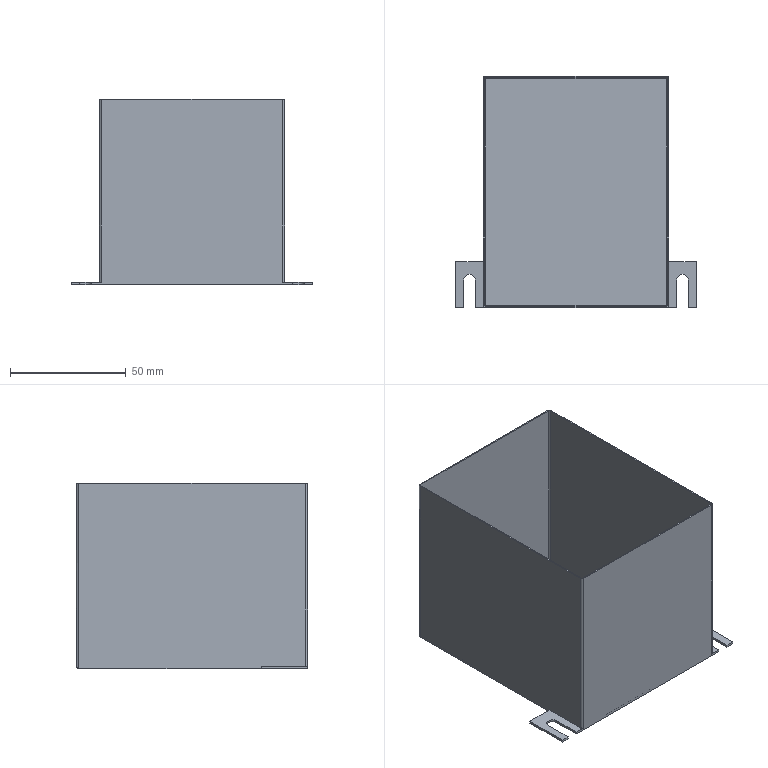Part | NX | features BREP 1 | 1 solid | 42 faces | box 104 x 100 x 80 mm | volume 18522 mm3 | plane 23 | cylinder 15 | sphere 4 | commonest cylinder face diameters 1 x8 2 x5 5 x2
STEP:
#1=CARTESIAN_POINT('',(48.5,-50.,0.));
#2=VERTEX_POINT('',#1);
#3=CARTESIAN_POINT('',(48.5,-50.,1.));
#4=VERTEX_POINT('',#3);
#5=CARTESIAN_POINT('',(48.5,-50.,-0.00005));
#6=DIRECTION('',(0.,0.,1.));
#7=VECTOR('',#6,1000.);
#8=LINE('',#5,#7);
#9=EDGE_CURVE('',#2,#4,#8,.T.);
#10=ORIENTED_EDGE('',*,*,#9,.F.);
#11=CARTESIAN_POINT('',(52.,-50.,0.));
#12=VERTEX_POINT('',#11);
#13=CARTESIAN_POINT('',(-40.,-50.,0.));
#14=DIRECTION('',(1.,0.,0.));
#15=VECTOR('',#14,1000.);
#16=LINE('',#13,#15);
#17=EDGE_CURVE('',#2,#12,#16,.T.);
#18=ORIENTED_EDGE('',*,*,#17,.T.);
#19=CARTESIAN_POINT('',(52.,-50.,1.));
#20=VERTEX_POINT('',#19);
#21=CARTESIAN_POINT('',(52.,-50.,0.));
#22=DIRECTION('',(0.,0.,1.));
#23=VECTOR('',#22,1000.);
#24=LINE('',#21,#23);
#25=EDGE_CURVE('',#12,#20,#24,.T.);
#26=ORIENTED_EDGE('',*,*,#25,.T.);
#27=CARTESIAN_POINT('',(52.,-50.,1.));
#28=DIRECTION('',(-1.,0.,0.));
#29=VECTOR('',#28,1000.);
#30=LINE('',#27,#29);
#31=EDGE_CURVE('',#20,#4,#30,.T.);
#32=ORIENTED_EDGE('',*,*,#31,.T.);
#33=EDGE_LOOP('',(#10,#18,#26,#32));
#34=FACE_BOUND('',#33,.T.);
#35=CARTESIAN_POINT('',(-40.,-50.,80.));
#36=DIRECTION('',(0.,1.,0.));
#37=DIRECTION('',(1.,0.,0.));
#38=AXIS2_PLACEMENT_3D('',#35,#36,#37);
#39=PLANE('',#38);
#40=ADVANCED_FACE('',(#34),#39,.F.);
#41=CARTESIAN_POINT('',(43.5,-50.,1.));
#42=VERTEX_POINT('',#41);
#43=CARTESIAN_POINT('',(39.,-50.,1.));
#44=VERTEX_POINT('',#43);
#45=CARTESIAN_POINT('',(52.,-50.,1.));
#46=DIRECTION('',(-1.,0.,0.));
#47=VECTOR('',#46,1000.);
#48=LINE('',#45,#47);
#49=EDGE_CURVE('',#42,#44,#48,.T.);
#50=ORIENTED_EDGE('',*,*,#49,.T.);
#51=CARTESIAN_POINT('',(39.,-50.,80.));
#52=VERTEX_POINT('',#51);
#53=CARTESIAN_POINT('',(39.,-50.,80.));
#54=DIRECTION('',(0.,0.,1.));
#55=VECTOR('',#54,1000.);
#56=LINE('',#53,#55);
#57=EDGE_CURVE('',#44,#52,#56,.T.);
#58=ORIENTED_EDGE('',*,*,#57,.T.);
#59=CARTESIAN_POINT('',(-39.,-50.,80.));
#60=VERTEX_POINT('',#59);
#61=CARTESIAN_POINT('',(-40.,-50.,80.));
#62=DIRECTION('',(1.,0.,0.));
#63=VECTOR('',#62,1000.);
#64=LINE('',#61,#63);
#65=EDGE_CURVE('',#60,#52,#64,.T.);
#66=ORIENTED_EDGE('',*,*,#65,.F.);
#67=CARTESIAN_POINT('',(-39.,-50.,1.));
#68=VERTEX_POINT('',#67);
#69=CARTESIAN_POINT('',(-39.,-50.,80.));
#70=DIRECTION('',(0.,0.,-1.));
#71=VECTOR('',#70,1000.);
#72=LINE('',#69,#71);
#73=EDGE_CURVE('',#60,#68,#72,.T.);
#74=ORIENTED_EDGE('',*,*,#73,.T.);
#75=CARTESIAN_POINT('',(-43.5,-50.,1.));
#76=VERTEX_POINT('',#75);
#77=CARTESIAN_POINT('',(-52.,-50.,1.));
#78=DIRECTION('',(1.,0.,0.));
#79=VECTOR('',#78,1000.);
#80=LINE('',#77,#79);
#81=EDGE_CURVE('',#76,#68,#80,.T.);
#82=ORIENTED_EDGE('',*,*,#81,.F.);
#83=CARTESIAN_POINT('',(-43.5,-50.,0.));
#84=VERTEX_POINT('',#83);
#85=CARTESIAN_POINT('',(-43.5,-50.,-0.00005));
#86=DIRECTION('',(0.,0.,1.));
#87=VECTOR('',#86,1000.);
#88=LINE('',#85,#87);
#89=EDGE_CURVE('',#84,#76,#88,.T.);
#90=ORIENTED_EDGE('',*,*,#89,.F.);
#91=CARTESIAN_POINT('',(43.5,-50.,0.));
#92=VERTEX_POINT('',#91);
#93=CARTESIAN_POINT('',(-40.,-50.,0.));
#94=DIRECTION('',(1.,0.,0.));
#95=VECTOR('',#94,1000.);
#96=LINE('',#93,#95);
#97=EDGE_CURVE('',#84,#92,#96,.T.);
#98=ORIENTED_EDGE('',*,*,#97,.T.);
#99=CARTESIAN_POINT('',(43.5,-50.,-0.00005));
#100=DIRECTION('',(0.,0.,1.));
#101=VECTOR('',#100,1000.);
#102=LINE('',#99,#101);
#103=EDGE_CURVE('',#92,#42,#102,.T.);
#104=ORIENTED_EDGE('',*,*,#103,.T.);
#105=EDGE_LOOP('',(#50,#58,#66,#74,#82,#90,#98,#104));
#106=FACE_BOUND('',#105,.T.);
#107=CARTESIAN_POINT('',(-40.,-50.,80.));
#108=DIRECTION('',(0.,1.,0.));
#109=DIRECTION('',(1.,0.,0.));
#110=AXIS2_PLACEMENT_3D('',#107,#108,#109);
#111=PLANE('',#110);
#112=ADVANCED_FACE('',(#106),#111,.F.);
#113=CARTESIAN_POINT('',(-40.,49.,0.));
#114=VERTEX_POINT('',#113);
#115=CARTESIAN_POINT('',(-40.,-30.,0.));
#116=VERTEX_POINT('',#115);
#117=CARTESIAN_POINT('',(-40.,-50.,0.));
#118=DIRECTION('',(0.,-1.,0.));
#119=VECTOR('',#118,1000.);
#120=LINE('',#117,#119);
#121=EDGE_CURVE('',#114,#116,#120,.T.);
#122=ORIENTED_EDGE('',*,*,#121,.F.);
#123=CARTESIAN_POINT('',(40.,49.,0.));
#124=VERTEX_POINT('',#123);
#125=CARTESIAN_POINT('',(40.,49.,0.));
#126=DIRECTION('',(1.,0.,0.));
#127=VECTOR('',#126,1000.);
#128=LINE('',#125,#127);
#129=EDGE_CURVE('',#114,#124,#128,.T.);
#130=ORIENTED_EDGE('',*,*,#129,.T.);
#131=CARTESIAN_POINT('',(40.,-30.,0.));
#132=VERTEX_POINT('',#131);
#133=CARTESIAN_POINT('',(40.,-50.,0.));
#134=DIRECTION('',(0.,1.,0.));
#135=VECTOR('',#134,1000.);
#136=LINE('',#133,#135);
#137=EDGE_CURVE('',#132,#124,#136,.T.);
#138=ORIENTED_EDGE('',*,*,#137,.F.);
#139=CARTESIAN_POINT('',(52.,-30.,0.));
#140=VERTEX_POINT('',#139);
#141=CARTESIAN_POINT('',(52.,-30.,0.));
#142=DIRECTION('',(-1.,0.,0.));
#143=VECTOR('',#142,1000.);
#144=LINE('',#141,#143);
#145=EDGE_CURVE('',#140,#132,#144,.T.);
#146=ORIENTED_EDGE('',*,*,#145,.F.);
#147=CARTESIAN_POINT('',(52.,-50.,0.));
#148=DIRECTION('',(0.,-1.,0.));
#149=VECTOR('',#148,1000.);
#150=LINE('',#147,#149);
#151=EDGE_CURVE('',#140,#12,#150,.T.);
#152=ORIENTED_EDGE('',*,*,#151,.T.);
#153=ORIENTED_EDGE('',*,*,#17,.F.);
#154=CARTESIAN_POINT('',(48.5,-38.,0.));
#155=VERTEX_POINT('',#154);
#156=CARTESIAN_POINT('',(48.5,0.,0.));
#157=DIRECTION('',(0.,1.,0.));
#158=VECTOR('',#157,1000.);
#159=LINE('',#156,#158);
#160=EDGE_CURVE('',#2,#155,#159,.T.);
#161=ORIENTED_EDGE('',*,*,#160,.T.);
#162=CARTESIAN_POINT('',(43.5,-38.,0.));
#163=VERTEX_POINT('',#162);
#164=CARTESIAN_POINT('',(46.,-38.,0.));
#165=DIRECTION('',(0.,0.,1.));
#166=DIRECTION('',(-1.,0.,0.));
#167=AXIS2_PLACEMENT_3D('',#164,#165,#166);
#168=CIRCLE('',#167,2.5);
#169=EDGE_CURVE('',#155,#163,#168,.T.);
#170=ORIENTED_EDGE('',*,*,#169,.T.);
#171=CARTESIAN_POINT('',(43.5,0.,0.));
#172=DIRECTION('',(0.,-1.,0.));
#173=VECTOR('',#172,1000.);
#174=LINE('',#171,#173);
#175=EDGE_CURVE('',#163,#92,#174,.T.);
#176=ORIENTED_EDGE('',*,*,#175,.T.);
#177=ORIENTED_EDGE('',*,*,#97,.F.);
#178=CARTESIAN_POINT('',(-43.5,-38.,0.));
#179=VERTEX_POINT('',#178);
#180=CARTESIAN_POINT('',(-43.5,0.,0.));
#181=DIRECTION('',(0.,-1.,0.));
#182=VECTOR('',#181,1000.);
#183=LINE('',#180,#182);
#184=EDGE_CURVE('',#179,#84,#183,.T.);
#185=ORIENTED_EDGE('',*,*,#184,.F.);
#186=CARTESIAN_POINT('',(-48.5,-38.,0.));
#187=VERTEX_POINT('',#186);
#188=CARTESIAN_POINT('',(-46.,-38.,0.));
#189=DIRECTION('',(0.,0.,-1.));
#190=DIRECTION('',(-1.,0.,0.));
#191=AXIS2_PLACEMENT_3D('',#188,#189,#190);
#192=CIRCLE('',#191,2.5);
#193=EDGE_CURVE('',#187,#179,#192,.T.);
#194=ORIENTED_EDGE('',*,*,#193,.F.);
#195=CARTESIAN_POINT('',(-48.5,-50.,0.));
#196=VERTEX_POINT('',#195);
#197=CARTESIAN_POINT('',(-48.5,0.,0.));
#198=DIRECTION('',(0.,1.,0.));
#199=VECTOR('',#198,1000.);
#200=LINE('',#197,#199);
#201=EDGE_CURVE('',#196,#187,#200,.T.);
#202=ORIENTED_EDGE('',*,*,#201,.F.);
#203=CARTESIAN_POINT('',(-52.,-50.,0.));
#204=VERTEX_POINT('',#203);
#205=CARTESIAN_POINT('',(-40.,-50.,0.));
#206=DIRECTION('',(1.,0.,0.));
#207=VECTOR('',#206,1000.);
#208=LINE('',#205,#207);
#209=EDGE_CURVE('',#204,#196,#208,.T.);
#210=ORIENTED_EDGE('',*,*,#209,.F.);
#211=CARTESIAN_POINT('',(-52.,-30.,0.));
#212=VERTEX_POINT('',#211);
#213=CARTESIAN_POINT('',(-52.,-50.,0.));
#214=DIRECTION('',(0.,-1.,0.));
#215=VECTOR('',#214,1000.);
#216=LINE('',#213,#215);
#217=EDGE_CURVE('',#212,#204,#216,.T.);
#218=ORIENTED_EDGE('',*,*,#217,.F.);
#219=CARTESIAN_POINT('',(-52.,-30.,0.));
#220=DIRECTION('',(1.,0.,0.));
#221=VECTOR('',#220,1000.);
#222=LINE('',#219,#221);
#223=EDGE_CURVE('',#212,#116,#222,.T.);
#224=ORIENTED_EDGE('',*,*,#223,.T.);
#225=EDGE_LOOP('',(#122,#130,#138,#146,#152,#153,#161,#170,#176,#177,#185,#194,#202,#210,#218,#224));
#226=FACE_BOUND('',#225,.T.);
#227=CARTESIAN_POINT('',(0.,0.,0.));
#228=DIRECTION('',(0.,0.,-1.));
#229=DIRECTION('',(0.,-1.,0.));
#230=AXIS2_PLACEMENT_3D('',#227,#228,#229);
#231=PLANE('',#230);
#232=ADVANCED_FACE('',(#226),#231,.T.);
#233=CARTESIAN_POINT('',(43.5,-38.,1.));
#234=VERTEX_POINT('',#233);
#235=CARTESIAN_POINT('',(48.5,-38.,1.));
#236=VERTEX_POINT('',#235);
#237=CARTESIAN_POINT('',(46.,-38.,1.));
#238=DIRECTION('',(0.,0.,-1.));
#239=DIRECTION('',(-1.,0.,0.));
#240=AXIS2_PLACEMENT_3D('',#237,#238,#239);
#241=CIRCLE('',#240,2.5);
#242=EDGE_CURVE('',#234,#236,#241,.T.);
#243=ORIENTED_EDGE('',*,*,#242,.T.);
#244=CARTESIAN_POINT('',(48.5,-38.,1.));
#245=DIRECTION('',(0.,-1.,0.));
#246=VECTOR('',#245,1000.);
#247=LINE('',#244,#246);
#248=EDGE_CURVE('',#236,#4,#247,.T.);
#249=ORIENTED_EDGE('',*,*,#248,.T.);
#250=ORIENTED_EDGE('',*,*,#31,.F.);
#251=CARTESIAN_POINT('',(52.,-30.,1.));
#252=VERTEX_POINT('',#251);
#253=CARTESIAN_POINT('',(52.,-50.,1.));
#254=DIRECTION('',(0.,1.,0.));
#255=VECTOR('',#254,1000.);
#256=LINE('',#253,#255);
#257=EDGE_CURVE('',#20,#252,#256,.T.);
#258=ORIENTED_EDGE('',*,*,#257,.T.);
#259=CARTESIAN_POINT('',(40.,-30.,1.));
#260=VERTEX_POINT('',#259);
#261=CARTESIAN_POINT('',(52.,-30.,1.));
#262=DIRECTION('',(-1.,0.,0.));
#263=VECTOR('',#262,1000.);
#264=LINE('',#261,#263);
#265=EDGE_CURVE('',#252,#260,#264,.T.);
#266=ORIENTED_EDGE('',*,*,#265,.T.);
#267=CARTESIAN_POINT('',(40.,-49.,1.));
#268=VERTEX_POINT('',#267);
#269=CARTESIAN_POINT('',(40.,-50.,1.));
#270=DIRECTION('',(0.,1.,0.));
#271=VECTOR('',#270,1000.);
#272=LINE('',#269,#271);
#273=EDGE_CURVE('',#268,#260,#272,.T.);
#274=ORIENTED_EDGE('',*,*,#273,.F.);
#275=CARTESIAN_POINT('',(39.,-49.,1.));
#276=DIRECTION('',(0.,0.,-1.));
#277=DIRECTION('',(1.,0.,0.));
#278=AXIS2_PLACEMENT_3D('',#275,#276,#277);
#279=CIRCLE('',#278,1.);
#280=EDGE_CURVE('',#268,#44,#279,.T.);
#281=ORIENTED_EDGE('',*,*,#280,.T.);
#282=ORIENTED_EDGE('',*,*,#49,.F.);
#283=CARTESIAN_POINT('',(43.5,-38.,1.));
#284=DIRECTION('',(0.,1.,0.));
#285=VECTOR('',#284,1000.);
#286=LINE('',#283,#285);
#287=EDGE_CURVE('',#42,#234,#286,.T.);
#288=ORIENTED_EDGE('',*,*,#287,.T.);
#289=EDGE_LOOP('',(#243,#249,#250,#258,#266,#274,#281,#282,#288));
#290=FACE_BOUND('',#289,.T.);
#291=CARTESIAN_POINT('',(52.,-50.,1.));
#292=DIRECTION('',(0.,0.,1.));
#293=DIRECTION('',(1.,0.,0.));
#294=AXIS2_PLACEMENT_3D('',#291,#292,#293);
#295=PLANE('',#294);
#296=ADVANCED_FACE('',(#290),#295,.T.);
#297=CARTESIAN_POINT('',(-40.,-49.,1.));
#298=VERTEX_POINT('',#297);
#299=CARTESIAN_POINT('',(-40.,-30.,1.));
#300=VERTEX_POINT('',#299);
#301=CARTESIAN_POINT('',(-40.,-50.,1.));
#302=DIRECTION('',(0.,1.,0.));
#303=VECTOR('',#302,1000.);
#304=LINE('',#301,#303);
#305=EDGE_CURVE('',#298,#300,#304,.T.);
#306=ORIENTED_EDGE('',*,*,#305,.F.);
#307=CARTESIAN_POINT('',(-40.,-49.,80.));
#308=VERTEX_POINT('',#307);
#309=CARTESIAN_POINT('',(-40.,-49.,80.));
#310=DIRECTION('',(0.,0.,1.));
#311=VECTOR('',#310,1000.);
#312=LINE('',#309,#311);
#313=EDGE_CURVE('',#298,#308,#312,.T.);
#314=ORIENTED_EDGE('',*,*,#313,.T.);
#315=CARTESIAN_POINT('',(-40.,49.,80.));
#316=VERTEX_POINT('',#315);
#317=CARTESIAN_POINT('',(-40.,-50.,80.));
#318=DIRECTION('',(0.,-1.,0.));
#319=VECTOR('',#318,1000.);
#320=LINE('',#317,#319);
#321=EDGE_CURVE('',#316,#308,#320,.T.);
#322=ORIENTED_EDGE('',*,*,#321,.F.);
#323=CARTESIAN_POINT('',(-40.,49.,80.));
#324=DIRECTION('',(0.,0.,-1.));
#325=VECTOR('',#324,1000.);
#326=LINE('',#323,#325);
#327=EDGE_CURVE('',#316,#114,#326,.T.);
#328=ORIENTED_EDGE('',*,*,#327,.T.);
#329=ORIENTED_EDGE('',*,*,#121,.T.);
#330=CARTESIAN_POINT('',(-40.,-30.,0.));
#331=DIRECTION('',(0.,0.,-1.));
#332=VECTOR('',#331,1000.);
#333=LINE('',#330,#332);
#334=EDGE_CURVE('',#300,#116,#333,.T.);
#335=ORIENTED_EDGE('',*,*,#334,.F.);
#336=EDGE_LOOP('',(#306,#314,#322,#328,#329,#335));
#337=FACE_BOUND('',#336,.T.);
#338=CARTESIAN_POINT('',(-40.,-50.,80.));
#339=DIRECTION('',(1.,0.,0.));
#340=DIRECTION('',(0.,1.,0.));
#341=AXIS2_PLACEMENT_3D('',#338,#339,#340);
#342=PLANE('',#341);
#343=ADVANCED_FACE('',(#337),#342,.F.);
#344=CARTESIAN_POINT('',(40.,-49.,80.));
#345=VERTEX_POINT('',#344);
#346=CARTESIAN_POINT('',(40.,49.,80.));
#347=VERTEX_POINT('',#346);
#348=CARTESIAN_POINT('',(40.,-50.,80.));
#349=DIRECTION('',(0.,1.,0.));
#350=VECTOR('',#349,1000.);
#351=LINE('',#348,#350);
#352=EDGE_CURVE('',#345,#347,#351,.T.);
#353=ORIENTED_EDGE('',*,*,#352,.T.);
#354=CARTESIAN_POINT('',(39.,50.,80.));
#355=VERTEX_POINT('',#354);
#356=CARTESIAN_POINT('',(39.,49.,80.));
#357=DIRECTION('',(0.,0.,1.));
#358=DIRECTION('',(-1.,0.,0.));
#359=AXIS2_PLACEMENT_3D('',#356,#357,#358);
#360=CIRCLE('',#359,1.);
#361=EDGE_CURVE('',#347,#355,#360,.T.);
#362=ORIENTED_EDGE('',*,*,#361,.T.);
#363=CARTESIAN_POINT('',(-39.,50.,80.));
#364=VERTEX_POINT('',#363);
#365=CARTESIAN_POINT('',(-40.,50.,80.));
#366=DIRECTION('',(-1.,0.,0.));
#367=VECTOR('',#366,1000.);
#368=LINE('',#365,#367);
#369=EDGE_CURVE('',#355,#364,#368,.T.);
#370=ORIENTED_EDGE('',*,*,#369,.T.);
#371=CARTESIAN_POINT('',(-39.,49.,80.));
#372=DIRECTION('',(0.,0.,1.));
#373=DIRECTION('',(-1.,0.,0.));
#374=AXIS2_PLACEMENT_3D('',#371,#372,#373);
#375=CIRCLE('',#374,1.);
#376=EDGE_CURVE('',#364,#316,#375,.T.);
#377=ORIENTED_EDGE('',*,*,#376,.T.);
#378=ORIENTED_EDGE('',*,*,#321,.T.);
#379=CARTESIAN_POINT('',(-39.,-49.,80.));
#380=DIRECTION('',(0.,0.,1.));
#381=DIRECTION('',(-1.,0.,0.));
#382=AXIS2_PLACEMENT_3D('',#379,#380,#381);
#383=CIRCLE('',#382,1.);
#384=EDGE_CURVE('',#308,#60,#383,.T.);
#385=ORIENTED_EDGE('',*,*,#384,.T.);
#386=ORIENTED_EDGE('',*,*,#65,.T.);
#387=CARTESIAN_POINT('',(39.,-49.,80.));
#388=DIRECTION('',(0.,0.,1.));
#389=DIRECTION('',(-1.,0.,0.));
#390=AXIS2_PLACEMENT_3D('',#387,#388,#389);
#391=CIRCLE('',#390,1.);
#392=EDGE_CURVE('',#52,#345,#391,.T.);
#393=ORIENTED_EDGE('',*,*,#392,.T.);
#394=EDGE_LOOP('',(#353,#362,#370,#377,#378,#385,#386,#393));
#395=FACE_BOUND('',#394,.T.);
#396=CARTESIAN_POINT('',(39.5,-49.,80.));
#397=VERTEX_POINT('',#396);
#398=CARTESIAN_POINT('',(39.5,49.,80.));
#399=VERTEX_POINT('',#398);
#400=CARTESIAN_POINT('',(39.5,0.,80.));
#401=DIRECTION('',(0.,1.,0.));
#402=VECTOR('',#401,1000.);
#403=LINE('',#400,#402);
#404=EDGE_CURVE('',#397,#399,#403,.T.);
#405=ORIENTED_EDGE('',*,*,#404,.F.);
#406=CARTESIAN_POINT('',(39.,-49.5,80.));
#407=VERTEX_POINT('',#406);
#408=CARTESIAN_POINT('',(39.,-49.,80.));
#409=DIRECTION('',(0.,0.,-1.));
#410=DIRECTION('',(-1.,0.,0.));
#411=AXIS2_PLACEMENT_3D('',#408,#409,#410);
#412=CIRCLE('',#411,0.5);
#413=EDGE_CURVE('',#397,#407,#412,.T.);
#414=ORIENTED_EDGE('',*,*,#413,.T.);
#415=CARTESIAN_POINT('',(-39.,-49.5,80.));
#416=VERTEX_POINT('',#415);
#417=CARTESIAN_POINT('',(0.,-49.5,80.));
#418=DIRECTION('',(1.,0.,0.));
#419=VECTOR('',#418,1000.);
#420=LINE('',#417,#419);
#421=EDGE_CURVE('',#416,#407,#420,.T.);
#422=ORIENTED_EDGE('',*,*,#421,.F.);
#423=CARTESIAN_POINT('',(-39.5,-49.,80.));
#424=VERTEX_POINT('',#423);
#425=CARTESIAN_POINT('',(-39.,-49.,80.));
#426=DIRECTION('',(0.,0.,-1.));
#427=DIRECTION('',(-1.,0.,0.));
#428=AXIS2_PLACEMENT_3D('',#425,#426,#427);
#429=CIRCLE('',#428,0.5);
#430=EDGE_CURVE('',#416,#424,#429,.T.);
#431=ORIENTED_EDGE('',*,*,#430,.T.);
#432=CARTESIAN_POINT('',(-39.5,49.,80.));
#433=VERTEX_POINT('',#432);
#434=CARTESIAN_POINT('',(-39.5,0.,80.));
#435=DIRECTION('',(0.,-1.,0.));
#436=VECTOR('',#435,1000.);
#437=LINE('',#434,#436);
#438=EDGE_CURVE('',#433,#424,#437,.T.);
#439=ORIENTED_EDGE('',*,*,#438,.F.);
#440=CARTESIAN_POINT('',(-39.,49.5,80.));
#441=VERTEX_POINT('',#440);
#442=CARTESIAN_POINT('',(-39.,49.,80.));
#443=DIRECTION('',(0.,0.,-1.));
#444=DIRECTION('',(-1.,0.,0.));
#445=AXIS2_PLACEMENT_3D('',#442,#443,#444);
#446=CIRCLE('',#445,0.5);
#447=EDGE_CURVE('',#433,#441,#446,.T.);
#448=ORIENTED_EDGE('',*,*,#447,.T.);
#449=CARTESIAN_POINT('',(39.,49.5,80.));
#450=VERTEX_POINT('',#449);
#451=CARTESIAN_POINT('',(0.,49.5,80.));
#452=DIRECTION('',(-1.,0.,0.));
#453=VECTOR('',#452,1000.);
#454=LINE('',#451,#453);
#455=EDGE_CURVE('',#450,#441,#454,.T.);
#456=ORIENTED_EDGE('',*,*,#455,.F.);
#457=CARTESIAN_POINT('',(39.,49.,80.));
#458=DIRECTION('',(0.,0.,-1.));
#459=DIRECTION('',(-1.,0.,0.));
#460=AXIS2_PLACEMENT_3D('',#457,#458,#459);
#461=CIRCLE('',#460,0.5);
#462=EDGE_CURVE('',#450,#399,#461,.T.);
#463=ORIENTED_EDGE('',*,*,#462,.T.);
#464=EDGE_LOOP('',(#405,#414,#422,#431,#439,#448,#456,#463));
#465=FACE_BOUND('',#464,.T.);
#466=CARTESIAN_POINT('',(0.,0.,80.));
#467=DIRECTION('',(0.,0.,-1.));
#468=DIRECTION('',(0.,-1.,0.));
#469=AXIS2_PLACEMENT_3D('',#466,#467,#468);
#470=PLANE('',#469);
#471=ADVANCED_FACE('',(#395,#465),#470,.F.);
#472=ORIENTED_EDGE('',*,*,#137,.T.);
#473=CARTESIAN_POINT('',(40.,49.,80.));
#474=DIRECTION('',(0.,0.,1.));
#475=VECTOR('',#474,1000.);
#476=LINE('',#473,#475);
#477=EDGE_CURVE('',#124,#347,#476,.T.);
#478=ORIENTED_EDGE('',*,*,#477,.T.);
#479=ORIENTED_EDGE('',*,*,#352,.F.);
#480=CARTESIAN_POINT('',(40.,-49.,80.));
#481=DIRECTION('',(0.,0.,-1.));
#482=VECTOR('',#481,1000.);
#483=LINE('',#480,#482);
#484=EDGE_CURVE('',#345,#268,#483,.T.);
#485=ORIENTED_EDGE('',*,*,#484,.T.);
#486=ORIENTED_EDGE('',*,*,#273,.T.);
#487=CARTESIAN_POINT('',(40.,-30.,0.));
#488=DIRECTION('',(0.,0.,-1.));
#489=VECTOR('',#488,1000.);
#490=LINE('',#487,#489);
#491=EDGE_CURVE('',#260,#132,#490,.T.);
#492=ORIENTED_EDGE('',*,*,#491,.T.);
#493=EDGE_LOOP('',(#472,#478,#479,#485,#486,#492));
#494=FACE_BOUND('',#493,.T.);
#495=CARTESIAN_POINT('',(40.,-50.,80.));
#496=DIRECTION('',(-1.,0.,0.));
#497=DIRECTION('',(0.,0.,1.));
#498=AXIS2_PLACEMENT_3D('',#495,#496,#497);
#499=PLANE('',#498);
#500=ADVANCED_FACE('',(#494),#499,.F.);
#501=ORIENTED_EDGE('',*,*,#369,.F.);
#502=CARTESIAN_POINT('',(39.,50.,1.));
#503=VERTEX_POINT('',#502);
#504=CARTESIAN_POINT('',(39.,50.,80.));
#505=DIRECTION('',(0.,0.,-1.));
#506=VECTOR('',#505,1000.);
#507=LINE('',#504,#506);
#508=EDGE_CURVE('',#355,#503,#507,.T.);
#509=ORIENTED_EDGE('',*,*,#508,.T.);
#510=CARTESIAN_POINT('',(-39.,50.,1.));
#511=VERTEX_POINT('',#510);
#512=CARTESIAN_POINT('',(-40.,50.,1.));
#513=DIRECTION('',(-1.,0.,0.));
#514=VECTOR('',#513,1000.);
#515=LINE('',#512,#514);
#516=EDGE_CURVE('',#503,#511,#515,.T.);
#517=ORIENTED_EDGE('',*,*,#516,.T.);
#518=CARTESIAN_POINT('',(-39.,50.,80.));
#519=DIRECTION('',(0.,0.,1.));
#520=VECTOR('',#519,1000.);
#521=LINE('',#518,#520);
#522=EDGE_CURVE('',#511,#364,#521,.T.);
#523=ORIENTED_EDGE('',*,*,#522,.T.);
#524=EDGE_LOOP('',(#501,#509,#517,#523));
#525=FACE_BOUND('',#524,.T.);
#526=CARTESIAN_POINT('',(-40.,50.,80.));
#527=DIRECTION('',(0.,-1.,0.));
#528=DIRECTION('',(0.,0.,-1.));
#529=AXIS2_PLACEMENT_3D('',#526,#527,#528);
#530=PLANE('',#529);
#531=ADVANCED_FACE('',(#525),#530,.F.);
#532=ORIENTED_EDGE('',*,*,#209,.T.);
#533=CARTESIAN_POINT('',(-48.5,-50.,1.));
#534=VERTEX_POINT('',#533);
#535=CARTESIAN_POINT('',(-48.5,-50.,-0.00005));
#536=DIRECTION('',(0.,0.,1.));
#537=VECTOR('',#536,1000.);
#538=LINE('',#535,#537);
#539=EDGE_CURVE('',#196,#534,#538,.T.);
#540=ORIENTED_EDGE('',*,*,#539,.T.);
#541=CARTESIAN_POINT('',(-52.,-50.,1.));
#542=VERTEX_POINT('',#541);
#543=CARTESIAN_POINT('',(-52.,-50.,1.));
#544=DIRECTION('',(1.,0.,0.));
#545=VECTOR('',#544,1000.);
#546=LINE('',#543,#545);
#547=EDGE_CURVE('',#542,#534,#546,.T.);
#548=ORIENTED_EDGE('',*,*,#547,.F.);
#549=CARTESIAN_POINT('',(-52.,-50.,0.));
#550=DIRECTION('',(0.,0.,1.));
#551=VECTOR('',#550,1000.);
#552=LINE('',#549,#551);
#553=EDGE_CURVE('',#204,#542,#552,.T.);
#554=ORIENTED_EDGE('',*,*,#553,.F.);
#555=EDGE_LOOP('',(#532,#540,#548,#554));
#556=FACE_BOUND('',#555,.T.);
#557=CARTESIAN_POINT('',(-40.,-50.,80.));
#558=DIRECTION('',(0.,1.,0.));
#559=DIRECTION('',(1.,0.,0.));
#560=AXIS2_PLACEMENT_3D('',#557,#558,#559);
#561=PLANE('',#560);
#562=ADVANCED_FACE('',(#556),#561,.F.);
#563=CARTESIAN_POINT('',(39.5,49.,1.));
#564=VERTEX_POINT('',#563);
#565=CARTESIAN_POINT('',(39.5,-49.,1.));
#566=VERTEX_POINT('',#565);
#567=CARTESIAN_POINT('',(39.5,-50.,1.));
#568=DIRECTION('',(0.,-1.,0.));
#569=VECTOR('',#568,1000.);
#570=LINE('',#567,#569);
#571=EDGE_CURVE('',#564,#566,#570,.T.);
#572=ORIENTED_EDGE('',*,*,#571,.T.);
#573=CARTESIAN_POINT('',(39.5,-49.,80.));
#574=DIRECTION('',(0.,0.,1.));
#575=VECTOR('',#574,1000.);
#576=LINE('',#573,#575);
#577=EDGE_CURVE('',#566,#397,#576,.T.);
#578=ORIENTED_EDGE('',*,*,#577,.T.);
#579=ORIENTED_EDGE('',*,*,#404,.T.);
#580=CARTESIAN_POINT('',(39.5,49.,0.5));
#581=DIRECTION('',(0.,0.,-1.));
#582=VECTOR('',#581,1000.);
#583=LINE('',#580,#582);
#584=EDGE_CURVE('',#399,#564,#583,.T.);
#585=ORIENTED_EDGE('',*,*,#584,.T.);
#586=EDGE_LOOP('',(#572,#578,#579,#585));
#587=FACE_BOUND('',#586,.T.);
#588=CARTESIAN_POINT('',(39.5,-50.,80.));
#589=DIRECTION('',(-1.,0.,0.));
#590=DIRECTION('',(0.,0.,1.));
#591=AXIS2_PLACEMENT_3D('',#588,#589,#590);
#592=PLANE('',#591);
#593=ADVANCED_FACE('',(#587),#592,.T.);
#594=ORIENTED_EDGE('',*,*,#455,.T.);
#595=CARTESIAN_POINT('',(-39.,49.5,1.));
#596=VERTEX_POINT('',#595);
#597=CARTESIAN_POINT('',(-39.,49.5,0.5));
#598=DIRECTION('',(0.,0.,-1.));
#599=VECTOR('',#598,1000.);
#600=LINE('',#597,#599);
#601=EDGE_CURVE('',#441,#596,#600,.T.);
#602=ORIENTED_EDGE('',*,*,#601,.T.);
#603=CARTESIAN_POINT('',(39.,49.5,1.));
#604=VERTEX_POINT('',#603);
#605=CARTESIAN_POINT('',(-40.,49.5,1.));
#606=DIRECTION('',(1.,0.,0.));
#607=VECTOR('',#606,1000.);
#608=LINE('',#605,#607);
#609=EDGE_CURVE('',#596,#604,#608,.T.);
#610=ORIENTED_EDGE('',*,*,#609,.T.);
#611=CARTESIAN_POINT('',(39.,49.5,80.));
#612=DIRECTION('',(0.,0.,1.));
#613=VECTOR('',#612,1000.);
#614=LINE('',#611,#613);
#615=EDGE_CURVE('',#604,#450,#614,.T.);
#616=ORIENTED_EDGE('',*,*,#615,.T.);
#617=EDGE_LOOP('',(#594,#602,#610,#616));
#618=FACE_BOUND('',#617,.T.);
#619=CARTESIAN_POINT('',(-40.,49.5,80.));
#620=DIRECTION('',(0.,-1.,0.));
#621=DIRECTION('',(0.,0.,-1.));
#622=AXIS2_PLACEMENT_3D('',#619,#620,#621);
#623=PLANE('',#622);
#624=ADVANCED_FACE('',(#618),#623,.T.);
#625=ORIENTED_EDGE('',*,*,#438,.T.);
#626=CARTESIAN_POINT('',(-39.5,-49.,1.));
#627=VERTEX_POINT('',#626);
#628=CARTESIAN_POINT('',(-39.5,-49.,0.5));
#629=DIRECTION('',(0.,0.,-1.));
#630=VECTOR('',#629,1000.);
#631=LINE('',#628,#630);
#632=EDGE_CURVE('',#424,#627,#631,.T.);
#633=ORIENTED_EDGE('',*,*,#632,.T.);
#634=CARTESIAN_POINT('',(-39.5,49.,1.));
#635=VERTEX_POINT('',#634);
#636=CARTESIAN_POINT('',(-39.5,-50.,1.));
#637=DIRECTION('',(0.,1.,0.));
#638=VECTOR('',#637,1000.);
#639=LINE('',#636,#638);
#640=EDGE_CURVE('',#627,#635,#639,.T.);
#641=ORIENTED_EDGE('',*,*,#640,.T.);
#642=CARTESIAN_POINT('',(-39.5,49.,80.));
#643=DIRECTION('',(0.,0.,1.));
#644=VECTOR('',#643,1000.);
#645=LINE('',#642,#644);
#646=EDGE_CURVE('',#635,#433,#645,.T.);
#647=ORIENTED_EDGE('',*,*,#646,.T.);
#648=EDGE_LOOP('',(#625,#633,#641,#647));
#649=FACE_BOUND('',#648,.T.);
#650=CARTESIAN_POINT('',(-39.5,-50.,80.));
#651=DIRECTION('',(1.,0.,0.));
#652=DIRECTION('',(0.,1.,0.));
#653=AXIS2_PLACEMENT_3D('',#650,#651,#652);
#654=PLANE('',#653);
#655=ADVANCED_FACE('',(#649),#654,.T.);
#656=ORIENTED_EDGE('',*,*,#421,.T.);
#657=CARTESIAN_POINT('',(39.,-49.5,1.));
#658=VERTEX_POINT('',#657);
#659=CARTESIAN_POINT('',(39.,-49.5,0.5));
#660=DIRECTION('',(0.,0.,-1.));
#661=VECTOR('',#660,1000.);
#662=LINE('',#659,#661);
#663=EDGE_CURVE('',#407,#658,#662,.T.);
#664=ORIENTED_EDGE('',*,*,#663,.T.);
#665=CARTESIAN_POINT('',(-39.,-49.5,1.));
#666=VERTEX_POINT('',#665);
#667=CARTESIAN_POINT('',(-40.,-49.5,1.));
#668=DIRECTION('',(-1.,0.,0.));
#669=VECTOR('',#668,1000.);
#670=LINE('',#667,#669);
#671=EDGE_CURVE('',#658,#666,#670,.T.);
#672=ORIENTED_EDGE('',*,*,#671,.T.);
#673=CARTESIAN_POINT('',(-39.,-49.5,80.));
#674=DIRECTION('',(0.,0.,1.));
#675=VECTOR('',#674,1000.);
#676=LINE('',#673,#675);
#677=EDGE_CURVE('',#666,#416,#676,.T.);
#678=ORIENTED_EDGE('',*,*,#677,.T.);
#679=EDGE_LOOP('',(#656,#664,#672,#678));
#680=FACE_BOUND('',#679,.T.);
#681=CARTESIAN_POINT('',(-40.,-49.5,80.));
#682=DIRECTION('',(0.,1.,0.));
#683=DIRECTION('',(1.,0.,0.));
#684=AXIS2_PLACEMENT_3D('',#681,#682,#683);
#685=PLANE('',#684);
#686=ADVANCED_FACE('',(#680),#685,.T.);
#687=CARTESIAN_POINT('',(-39.,49.,0.5));
#688=VERTEX_POINT('',#687);
#689=CARTESIAN_POINT('',(-39.,-49.,0.5));
#690=VERTEX_POINT('',#689);
#691=CARTESIAN_POINT('',(-39.,0.,0.5));
#692=DIRECTION('',(0.,-1.,0.));
#693=VECTOR('',#692,1000.);
#694=LINE('',#691,#693);
#695=EDGE_CURVE('',#688,#690,#694,.T.);
#696=ORIENTED_EDGE('',*,*,#695,.T.);
#697=CARTESIAN_POINT('',(39.,-49.,0.5));
#698=VERTEX_POINT('',#697);
#699=CARTESIAN_POINT('',(0.,-49.,0.5));
#700=DIRECTION('',(1.,0.,0.));
#701=VECTOR('',#700,1000.);
#702=LINE('',#699,#701);
#703=EDGE_CURVE('',#690,#698,#702,.T.);
#704=ORIENTED_EDGE('',*,*,#703,.T.);
#705=CARTESIAN_POINT('',(39.,49.,0.5));
#706=VERTEX_POINT('',#705);
#707=CARTESIAN_POINT('',(39.,0.,0.5));
#708=DIRECTION('',(0.,1.,0.));
#709=VECTOR('',#708,1000.);
#710=LINE('',#707,#709);
#711=EDGE_CURVE('',#698,#706,#710,.T.);
#712=ORIENTED_EDGE('',*,*,#711,.T.);
#713=CARTESIAN_POINT('',(0.,49.,0.5));
#714=DIRECTION('',(-1.,0.,0.));
#715=VECTOR('',#714,1000.);
#716=LINE('',#713,#715);
#717=EDGE_CURVE('',#706,#688,#716,.T.);
#718=ORIENTED_EDGE('',*,*,#717,.T.);
#719=EDGE_LOOP('',(#696,#704,#712,#718));
#720=FACE_BOUND('',#719,.T.);
#721=CARTESIAN_POINT('',(0.,0.,0.5));
#722=DIRECTION('',(0.,0.,-1.));
#723=DIRECTION('',(0.,-1.,0.));
#724=AXIS2_PLACEMENT_3D('',#721,#722,#723);
#725=PLANE('',#724);
#726=ADVANCED_FACE('',(#720),#725,.F.);
#727=CARTESIAN_POINT('',(-43.5,-38.,1.));
#728=VERTEX_POINT('',#727);
#729=CARTESIAN_POINT('',(-48.5,-38.,1.));
#730=VERTEX_POINT('',#729);
#731=CARTESIAN_POINT('',(-46.,-38.,1.));
#732=DIRECTION('',(0.,0.,1.));
#733=DIRECTION('',(1.,0.,0.));
#734=AXIS2_PLACEMENT_3D('',#731,#732,#733);
#735=CIRCLE('',#734,2.5);
#736=EDGE_CURVE('',#728,#730,#735,.T.);
#737=ORIENTED_EDGE('',*,*,#736,.F.);
#738=CARTESIAN_POINT('',(-43.5,-38.,1.));
#739=DIRECTION('',(0.,1.,0.));
#740=VECTOR('',#739,1000.);
#741=LINE('',#738,#740);
#742=EDGE_CURVE('',#76,#728,#741,.T.);
#743=ORIENTED_EDGE('',*,*,#742,.F.);
#744=ORIENTED_EDGE('',*,*,#81,.T.);
#745=CARTESIAN_POINT('',(-39.,-49.,1.));
#746=DIRECTION('',(0.,0.,-1.));
#747=DIRECTION('',(-1.,0.,0.));
#748=AXIS2_PLACEMENT_3D('',#745,#746,#747);
#749=CIRCLE('',#748,1.);
#750=EDGE_CURVE('',#68,#298,#749,.T.);
#751=ORIENTED_EDGE('',*,*,#750,.T.);
#752=ORIENTED_EDGE('',*,*,#305,.T.);
#753=CARTESIAN_POINT('',(-52.,-30.,1.));
#754=VERTEX_POINT('',#753);
#755=CARTESIAN_POINT('',(-52.,-30.,1.));
#756=DIRECTION('',(1.,0.,0.));
#757=VECTOR('',#756,1000.);
#758=LINE('',#755,#757);
#759=EDGE_CURVE('',#754,#300,#758,.T.);
#760=ORIENTED_EDGE('',*,*,#759,.F.);
#761=CARTESIAN_POINT('',(-52.,-50.,1.));
#762=DIRECTION('',(0.,1.,0.));
#763=VECTOR('',#762,1000.);
#764=LINE('',#761,#763);
#765=EDGE_CURVE('',#542,#754,#764,.T.);
#766=ORIENTED_EDGE('',*,*,#765,.F.);
#767=ORIENTED_EDGE('',*,*,#547,.T.);
#768=CARTESIAN_POINT('',(-48.5,-38.,1.));
#769=DIRECTION('',(0.,-1.,0.));
#770=VECTOR('',#769,1000.);
#771=LINE('',#768,#770);
#772=EDGE_CURVE('',#730,#534,#771,.T.);
#773=ORIENTED_EDGE('',*,*,#772,.F.);
#774=EDGE_LOOP('',(#737,#743,#744,#751,#752,#760,#766,#767,#773));
#775=FACE_BOUND('',#774,.T.);
#776=CARTESIAN_POINT('',(-52.,-50.,1.));
#777=DIRECTION('',(0.,0.,-1.));
#778=DIRECTION('',(0.,-1.,0.));
#779=AXIS2_PLACEMENT_3D('',#776,#777,#778);
#780=PLANE('',#779);
#781=ADVANCED_FACE('',(#775),#780,.F.);
#782=ORIENTED_EDGE('',*,*,#334,.T.);
#783=ORIENTED_EDGE('',*,*,#223,.F.);
#784=CARTESIAN_POINT('',(-52.,-30.,0.));
#785=DIRECTION('',(0.,0.,-1.));
#786=VECTOR('',#785,1000.);
#787=LINE('',#784,#786);
#788=EDGE_CURVE('',#754,#212,#787,.T.);
#789=ORIENTED_EDGE('',*,*,#788,.F.);
#790=ORIENTED_EDGE('',*,*,#759,.T.);
#791=EDGE_LOOP('',(#782,#783,#789,#790));
#792=FACE_BOUND('',#791,.T.);
#793=CARTESIAN_POINT('',(-52.,-30.,0.));
#794=DIRECTION('',(0.,-1.,0.));
#795=DIRECTION('',(0.,0.,-1.));
#796=AXIS2_PLACEMENT_3D('',#793,#794,#795);
#797=PLANE('',#796);
#798=ADVANCED_FACE('',(#792),#797,.F.);
#799=ORIENTED_EDGE('',*,*,#217,.T.);
#800=ORIENTED_EDGE('',*,*,#553,.T.);
#801=ORIENTED_EDGE('',*,*,#765,.T.);
#802=ORIENTED_EDGE('',*,*,#788,.T.);
#803=EDGE_LOOP('',(#799,#800,#801,#802));
#804=FACE_BOUND('',#803,.T.);
#805=CARTESIAN_POINT('',(-52.,0.,0.));
#806=DIRECTION('',(1.,0.,0.));
#807=DIRECTION('',(0.,1.,0.));
#808=AXIS2_PLACEMENT_3D('',#805,#806,#807);
#809=PLANE('',#808);
#810=ADVANCED_FACE('',(#804),#809,.F.);
#811=ORIENTED_EDGE('',*,*,#193,.T.);
#812=CARTESIAN_POINT('',(-43.5,-38.,-0.00005));
#813=DIRECTION('',(0.,0.,1.));
#814=VECTOR('',#813,1000.);
#815=LINE('',#812,#814);
#816=EDGE_CURVE('',#179,#728,#815,.T.);
#817=ORIENTED_EDGE('',*,*,#816,.T.);
#818=ORIENTED_EDGE('',*,*,#736,.T.);
#819=CARTESIAN_POINT('',(-48.5,-38.,-0.00005));
#820=DIRECTION('',(0.,0.,1.));
#821=VECTOR('',#820,1000.);
#822=LINE('',#819,#821);
#823=EDGE_CURVE('',#187,#730,#822,.T.);
#824=ORIENTED_EDGE('',*,*,#823,.F.);
#825=EDGE_LOOP('',(#811,#817,#818,#824));
#826=FACE_BOUND('',#825,.T.);
#827=CARTESIAN_POINT('',(-46.,-38.,-0.00005));
#828=DIRECTION('',(0.,0.,1.));
#829=DIRECTION('',(1.,0.,0.));
#830=AXIS2_PLACEMENT_3D('',#827,#828,#829);
#831=CYLINDRICAL_SURFACE('',#830,2.5);
#832=ADVANCED_FACE('',(#826),#831,.F.);
#833=ORIENTED_EDGE('',*,*,#184,.T.);
#834=ORIENTED_EDGE('',*,*,#89,.T.);
#835=ORIENTED_EDGE('',*,*,#742,.T.);
#836=ORIENTED_EDGE('',*,*,#816,.F.);
#837=EDGE_LOOP('',(#833,#834,#835,#836));
#838=FACE_BOUND('',#837,.T.);
#839=CARTESIAN_POINT('',(-43.5,-38.,-0.00005));
#840=DIRECTION('',(1.,0.,0.));
#841=DIRECTION('',(0.,1.,0.));
#842=AXIS2_PLACEMENT_3D('',#839,#840,#841);
#843=PLANE('',#842);
#844=ADVANCED_FACE('',(#838),#843,.F.);
#845=ORIENTED_EDGE('',*,*,#201,.T.);
#846=ORIENTED_EDGE('',*,*,#823,.T.);
#847=ORIENTED_EDGE('',*,*,#772,.T.);
#848=ORIENTED_EDGE('',*,*,#539,.F.);
#849=EDGE_LOOP('',(#845,#846,#847,#848));
#850=FACE_BOUND('',#849,.T.);
#851=CARTESIAN_POINT('',(-48.5,-38.,-0.00005));
#852=DIRECTION('',(-1.,0.,0.));
#853=DIRECTION('',(0.,1.,0.));
#854=AXIS2_PLACEMENT_3D('',#851,#852,#853);
#855=PLANE('',#854);
#856=ADVANCED_FACE('',(#850),#855,.F.);
#857=ORIENTED_EDGE('',*,*,#491,.F.);
#858=ORIENTED_EDGE('',*,*,#265,.F.);
#859=CARTESIAN_POINT('',(52.,-30.,0.));
#860=DIRECTION('',(0.,0.,-1.));
#861=VECTOR('',#860,1000.);
#862=LINE('',#859,#861);
#863=EDGE_CURVE('',#252,#140,#862,.T.);
#864=ORIENTED_EDGE('',*,*,#863,.T.);
#865=ORIENTED_EDGE('',*,*,#145,.T.);
#866=EDGE_LOOP('',(#857,#858,#864,#865));
#867=FACE_BOUND('',#866,.T.);
#868=CARTESIAN_POINT('',(52.,-30.,0.));
#869=DIRECTION('',(0.,1.,0.));
#870=DIRECTION('',(1.,0.,0.));
#871=AXIS2_PLACEMENT_3D('',#868,#869,#870);
#872=PLANE('',#871);
#873=ADVANCED_FACE('',(#867),#872,.T.);
#874=ORIENTED_EDGE('',*,*,#151,.F.);
#875=ORIENTED_EDGE('',*,*,#863,.F.);
#876=ORIENTED_EDGE('',*,*,#257,.F.);
#877=ORIENTED_EDGE('',*,*,#25,.F.);
#878=EDGE_LOOP('',(#874,#875,#876,#877));
#879=FACE_BOUND('',#878,.T.);
#880=CARTESIAN_POINT('',(52.,0.,0.));
#881=DIRECTION('',(-1.,0.,0.));
#882=DIRECTION('',(0.,0.,1.));
#883=AXIS2_PLACEMENT_3D('',#880,#881,#882);
#884=PLANE('',#883);
#885=ADVANCED_FACE('',(#879),#884,.F.);
#886=CARTESIAN_POINT('',(48.5,-38.,-0.00005));
#887=DIRECTION('',(0.,0.,1.));
#888=VECTOR('',#887,1000.);
#889=LINE('',#886,#888);
#890=EDGE_CURVE('',#155,#236,#889,.T.);
#891=ORIENTED_EDGE('',*,*,#890,.T.);
#892=ORIENTED_EDGE('',*,*,#242,.F.);
#893=CARTESIAN_POINT('',(43.5,-38.,-0.00005));
#894=DIRECTION('',(0.,0.,1.));
#895=VECTOR('',#894,1000.);
#896=LINE('',#893,#895);
#897=EDGE_CURVE('',#163,#234,#896,.T.);
#898=ORIENTED_EDGE('',*,*,#897,.F.);
#899=ORIENTED_EDGE('',*,*,#169,.F.);
#900=EDGE_LOOP('',(#891,#892,#898,#899));
#901=FACE_BOUND('',#900,.T.);
#902=CARTESIAN_POINT('',(46.,-38.,-0.00005));
#903=DIRECTION('',(0.,0.,1.));
#904=DIRECTION('',(1.,0.,0.));
#905=AXIS2_PLACEMENT_3D('',#902,#903,#904);
#906=CYLINDRICAL_SURFACE('',#905,2.5);
#907=ADVANCED_FACE('',(#901),#906,.F.);
#908=ORIENTED_EDGE('',*,*,#9,.T.);
#909=ORIENTED_EDGE('',*,*,#248,.F.);
#910=ORIENTED_EDGE('',*,*,#890,.F.);
#911=ORIENTED_EDGE('',*,*,#160,.F.);
#912=EDGE_LOOP('',(#908,#909,#910,#911));
#913=FACE_BOUND('',#912,.T.);
#914=CARTESIAN_POINT('',(48.5,-38.,-0.00005));
#915=DIRECTION('',(-1.,0.,0.));
#916=DIRECTION('',(0.,0.,1.));
#917=AXIS2_PLACEMENT_3D('',#914,#915,#916);
#918=PLANE('',#917);
#919=ADVANCED_FACE('',(#913),#918,.T.);
#920=ORIENTED_EDGE('',*,*,#897,.T.);
#921=ORIENTED_EDGE('',*,*,#287,.F.);
#922=ORIENTED_EDGE('',*,*,#103,.F.);
#923=ORIENTED_EDGE('',*,*,#175,.F.);
#924=EDGE_LOOP('',(#920,#921,#922,#923));
#925=FACE_BOUND('',#924,.T.);
#926=CARTESIAN_POINT('',(43.5,-38.,-0.00005));
#927=DIRECTION('',(1.,0.,0.));
#928=DIRECTION('',(0.,-1.,0.));
#929=AXIS2_PLACEMENT_3D('',#926,#927,#928);
#930=PLANE('',#929);
#931=ADVANCED_FACE('',(#925),#930,.T.);
#932=CARTESIAN_POINT('',(-39.,49.,1.));
#933=DIRECTION('',(0.,0.,1.));
#934=DIRECTION('',(1.,0.,0.));
#935=AXIS2_PLACEMENT_3D('',#932,#933,#934);
#936=CIRCLE('',#935,0.5);
#937=EDGE_CURVE('',#596,#635,#936,.T.);
#938=ORIENTED_EDGE('',*,*,#937,.F.);
#939=ORIENTED_EDGE('',*,*,#601,.F.);
#940=ORIENTED_EDGE('',*,*,#447,.F.);
#941=ORIENTED_EDGE('',*,*,#646,.F.);
#942=EDGE_LOOP('',(#938,#939,#940,#941));
#943=FACE_BOUND('',#942,.T.);
#944=CARTESIAN_POINT('',(-39.,49.,80.));
#945=DIRECTION('',(0.,0.,1.));
#946=DIRECTION('',(1.,0.,0.));
#947=AXIS2_PLACEMENT_3D('',#944,#945,#946);
#948=CYLINDRICAL_SURFACE('',#947,0.5);
#949=ADVANCED_FACE('',(#943),#948,.F.);
#950=CARTESIAN_POINT('',(-39.,49.,1.));
#951=DIRECTION('',(-1.,0.,0.));
#952=DIRECTION('',(0.,0.,-1.));
#953=AXIS2_PLACEMENT_3D('',#950,#951,#952);
#954=CIRCLE('',#953,0.5);
#955=EDGE_CURVE('',#596,#688,#954,.T.);
#956=ORIENTED_EDGE('',*,*,#955,.F.);
#957=ORIENTED_EDGE('',*,*,#937,.T.);
#958=CARTESIAN_POINT('',(-39.,49.,1.));
#959=DIRECTION('',(0.,1.,0.));
#960=DIRECTION('',(0.,0.,-1.));
#961=AXIS2_PLACEMENT_3D('',#958,#959,#960);
#962=CIRCLE('',#961,0.5);
#963=EDGE_CURVE('',#688,#635,#962,.T.);
#964=ORIENTED_EDGE('',*,*,#963,.F.);
#965=EDGE_LOOP('',(#956,#957,#964));
#966=FACE_BOUND('',#965,.T.);
#967=CARTESIAN_POINT('',(-39.,49.,1.));
#968=DIRECTION('',(0.,0.,-1.));
#969=DIRECTION('',(1.,0.,0.));
#970=AXIS2_PLACEMENT_3D('',#967,#968,#969);
#971=SPHERICAL_SURFACE('',#970,0.5);
#972=ADVANCED_FACE('',(#966),#971,.F.);
#973=ORIENTED_EDGE('',*,*,#430,.F.);
#974=ORIENTED_EDGE('',*,*,#677,.F.);
#975=CARTESIAN_POINT('',(-39.,-49.,1.));
#976=DIRECTION('',(0.,0.,1.));
#977=DIRECTION('',(1.,0.,0.));
#978=AXIS2_PLACEMENT_3D('',#975,#976,#977);
#979=CIRCLE('',#978,0.5);
#980=EDGE_CURVE('',#627,#666,#979,.T.);
#981=ORIENTED_EDGE('',*,*,#980,.F.);
#982=ORIENTED_EDGE('',*,*,#632,.F.);
#983=EDGE_LOOP('',(#973,#974,#981,#982));
#984=FACE_BOUND('',#983,.T.);
#985=CARTESIAN_POINT('',(-39.,-49.,80.));
#986=DIRECTION('',(0.,0.,1.));
#987=DIRECTION('',(1.,0.,0.));
#988=AXIS2_PLACEMENT_3D('',#985,#986,#987);
#989=CYLINDRICAL_SURFACE('',#988,0.5);
#990=ADVANCED_FACE('',(#984),#989,.F.);
#991=ORIENTED_EDGE('',*,*,#963,.T.);
#992=ORIENTED_EDGE('',*,*,#640,.F.);
#993=CARTESIAN_POINT('',(-39.,-49.,1.));
#994=DIRECTION('',(0.,1.,0.));
#995=DIRECTION('',(0.,0.,1.));
#996=AXIS2_PLACEMENT_3D('',#993,#994,#995);
#997=CIRCLE('',#996,0.5);
#998=EDGE_CURVE('',#690,#627,#997,.T.);
#999=ORIENTED_EDGE('',*,*,#998,.F.);
#1000=ORIENTED_EDGE('',*,*,#695,.F.);
#1001=EDGE_LOOP('',(#991,#992,#999,#1000));
#1002=FACE_BOUND('',#1001,.T.);
#1003=CARTESIAN_POINT('',(-39.,0.,1.));
#1004=DIRECTION('',(0.,-1.,0.));
#1005=DIRECTION('',(0.,0.,-1.));
#1006=AXIS2_PLACEMENT_3D('',#1003,#1004,#1005);
#1007=CYLINDRICAL_SURFACE('',#1006,0.5);
#1008=ADVANCED_FACE('',(#1002),#1007,.F.);
#1009=ORIENTED_EDGE('',*,*,#955,.T.);
#1010=ORIENTED_EDGE('',*,*,#717,.F.);
#1011=CARTESIAN_POINT('',(39.,49.,1.));
#1012=DIRECTION('',(-1.,0.,0.));
#1013=DIRECTION('',(0.,0.,1.));
#1014=AXIS2_PLACEMENT_3D('',#1011,#1012,#1013);
#1015=CIRCLE('',#1014,0.5);
#1016=EDGE_CURVE('',#604,#706,#1015,.T.);
#1017=ORIENTED_EDGE('',*,*,#1016,.F.);
#1018=ORIENTED_EDGE('',*,*,#609,.F.);
#1019=EDGE_LOOP('',(#1009,#1010,#1017,#1018));
#1020=FACE_BOUND('',#1019,.T.);
#1021=CARTESIAN_POINT('',(0.,49.,1.));
#1022=DIRECTION('',(-1.,0.,0.));
#1023=DIRECTION('',(0.,0.,1.));
#1024=AXIS2_PLACEMENT_3D('',#1021,#1022,#1023);
#1025=CYLINDRICAL_SURFACE('',#1024,0.5);
#1026=ADVANCED_FACE('',(#1020),#1025,.F.);
#1027=ORIENTED_EDGE('',*,*,#462,.F.);
#1028=ORIENTED_EDGE('',*,*,#615,.F.);
#1029=CARTESIAN_POINT('',(39.,49.,1.));
#1030=DIRECTION('',(0.,0.,1.));
#1031=DIRECTION('',(1.,0.,0.));
#1032=AXIS2_PLACEMENT_3D('',#1029,#1030,#1031);
#1033=CIRCLE('',#1032,0.5);
#1034=EDGE_CURVE('',#564,#604,#1033,.T.);
#1035=ORIENTED_EDGE('',*,*,#1034,.F.);
#1036=ORIENTED_EDGE('',*,*,#584,.F.);
#1037=EDGE_LOOP('',(#1027,#1028,#1035,#1036));
#1038=FACE_BOUND('',#1037,.T.);
#1039=CARTESIAN_POINT('',(39.,49.,80.));
#1040=DIRECTION('',(0.,0.,1.));
#1041=DIRECTION('',(1.,0.,0.));
#1042=AXIS2_PLACEMENT_3D('',#1039,#1040,#1041);
#1043=CYLINDRICAL_SURFACE('',#1042,0.5);
#1044=ADVANCED_FACE('',(#1038),#1043,.F.);
#1045=ORIENTED_EDGE('',*,*,#998,.T.);
#1046=ORIENTED_EDGE('',*,*,#980,.T.);
#1047=CARTESIAN_POINT('',(-39.,-49.,1.));
#1048=DIRECTION('',(-1.,0.,0.));
#1049=DIRECTION('',(0.,0.,-1.));
#1050=AXIS2_PLACEMENT_3D('',#1047,#1048,#1049);
#1051=CIRCLE('',#1050,0.5);
#1052=EDGE_CURVE('',#690,#666,#1051,.T.);
#1053=ORIENTED_EDGE('',*,*,#1052,.F.);
#1054=EDGE_LOOP('',(#1045,#1046,#1053));
#1055=FACE_BOUND('',#1054,.T.);
#1056=CARTESIAN_POINT('',(-39.,-49.,1.));
#1057=DIRECTION('',(0.,0.,-1.));
#1058=DIRECTION('',(1.,0.,0.));
#1059=AXIS2_PLACEMENT_3D('',#1056,#1057,#1058);
#1060=SPHERICAL_SURFACE('',#1059,0.5);
#1061=ADVANCED_FACE('',(#1055),#1060,.F.);
#1062=ORIENTED_EDGE('',*,*,#1034,.T.);
#1063=ORIENTED_EDGE('',*,*,#1016,.T.);
#1064=CARTESIAN_POINT('',(39.,49.,1.));
#1065=DIRECTION('',(0.,1.,0.));
#1066=DIRECTION('',(0.,0.,-1.));
#1067=AXIS2_PLACEMENT_3D('',#1064,#1065,#1066);
#1068=CIRCLE('',#1067,0.5);
#1069=EDGE_CURVE('',#564,#706,#1068,.T.);
#1070=ORIENTED_EDGE('',*,*,#1069,.F.);
#1071=EDGE_LOOP('',(#1062,#1063,#1070));
#1072=FACE_BOUND('',#1071,.T.);
#1073=CARTESIAN_POINT('',(39.,49.,1.));
#1074=DIRECTION('',(0.,0.,-1.));
#1075=DIRECTION('',(1.,0.,0.));
#1076=AXIS2_PLACEMENT_3D('',#1073,#1074,#1075);
#1077=SPHERICAL_SURFACE('',#1076,0.5);
#1078=ADVANCED_FACE('',(#1072),#1077,.F.);
#1079=ORIENTED_EDGE('',*,*,#1052,.T.);
#1080=ORIENTED_EDGE('',*,*,#671,.F.);
#1081=CARTESIAN_POINT('',(39.,-49.,1.));
#1082=DIRECTION('',(-1.,0.,0.));
#1083=DIRECTION('',(0.,0.,1.));
#1084=AXIS2_PLACEMENT_3D('',#1081,#1082,#1083);
#1085=CIRCLE('',#1084,0.5);
#1086=EDGE_CURVE('',#698,#658,#1085,.T.);
#1087=ORIENTED_EDGE('',*,*,#1086,.F.);
#1088=ORIENTED_EDGE('',*,*,#703,.F.);
#1089=EDGE_LOOP('',(#1079,#1080,#1087,#1088));
#1090=FACE_BOUND('',#1089,.T.);
#1091=CARTESIAN_POINT('',(0.,-49.,1.));
#1092=DIRECTION('',(1.,0.,0.));
#1093=DIRECTION('',(0.,0.,-1.));
#1094=AXIS2_PLACEMENT_3D('',#1091,#1092,#1093);
#1095=CYLINDRICAL_SURFACE('',#1094,0.5);
#1096=ADVANCED_FACE('',(#1090),#1095,.F.);
#1097=ORIENTED_EDGE('',*,*,#1069,.T.);
#1098=ORIENTED_EDGE('',*,*,#711,.F.);
#1099=CARTESIAN_POINT('',(39.,-49.,1.));
#1100=DIRECTION('',(0.,1.,0.));
#1101=DIRECTION('',(0.,0.,1.));
#1102=AXIS2_PLACEMENT_3D('',#1099,#1100,#1101);
#1103=CIRCLE('',#1102,0.5);
#1104=EDGE_CURVE('',#566,#698,#1103,.T.);
#1105=ORIENTED_EDGE('',*,*,#1104,.F.);
#1106=ORIENTED_EDGE('',*,*,#571,.F.);
#1107=EDGE_LOOP('',(#1097,#1098,#1105,#1106));
#1108=FACE_BOUND('',#1107,.T.);
#1109=CARTESIAN_POINT('',(39.,0.,1.));
#1110=DIRECTION('',(0.,1.,0.));
#1111=DIRECTION('',(0.,0.,1.));
#1112=AXIS2_PLACEMENT_3D('',#1109,#1110,#1111);
#1113=CYLINDRICAL_SURFACE('',#1112,0.5);
#1114=ADVANCED_FACE('',(#1108),#1113,.F.);
#1115=ORIENTED_EDGE('',*,*,#1104,.T.);
#1116=ORIENTED_EDGE('',*,*,#1086,.T.);
#1117=CARTESIAN_POINT('',(39.,-49.,1.));
#1118=DIRECTION('',(0.,0.,-1.));
#1119=DIRECTION('',(1.,0.,0.));
#1120=AXIS2_PLACEMENT_3D('',#1117,#1118,#1119);
#1121=CIRCLE('',#1120,0.5);
#1122=EDGE_CURVE('',#566,#658,#1121,.T.);
#1123=ORIENTED_EDGE('',*,*,#1122,.F.);
#1124=EDGE_LOOP('',(#1115,#1116,#1123));
#1125=FACE_BOUND('',#1124,.T.);
#1126=CARTESIAN_POINT('',(39.,-49.,1.));
#1127=DIRECTION('',(0.,0.,-1.));
#1128=DIRECTION('',(1.,0.,0.));
#1129=AXIS2_PLACEMENT_3D('',#1126,#1127,#1128);
#1130=SPHERICAL_SURFACE('',#1129,0.5);
#1131=ADVANCED_FACE('',(#1125),#1130,.F.);
#1132=ORIENTED_EDGE('',*,*,#413,.F.);
#1133=ORIENTED_EDGE('',*,*,#577,.F.);
#1134=ORIENTED_EDGE('',*,*,#1122,.T.);
#1135=ORIENTED_EDGE('',*,*,#663,.F.);
#1136=EDGE_LOOP('',(#1132,#1133,#1134,#1135));
#1137=FACE_BOUND('',#1136,.T.);
#1138=CARTESIAN_POINT('',(39.,-49.,80.));
#1139=DIRECTION('',(0.,0.,1.));
#1140=DIRECTION('',(1.,0.,0.));
#1141=AXIS2_PLACEMENT_3D('',#1138,#1139,#1140);
#1142=CYLINDRICAL_SURFACE('',#1141,0.5);
#1143=ADVANCED_FACE('',(#1137),#1142,.F.);
#1144=ORIENTED_EDGE('',*,*,#361,.F.);
#1145=ORIENTED_EDGE('',*,*,#477,.F.);
#1146=CARTESIAN_POINT('',(39.,50.,1.));
#1147=CARTESIAN_POINT('',(39.586,50.,0.4142));
#1148=CARTESIAN_POINT('',(40.,49.586,0.));
#1149=CARTESIAN_POINT('',(40.,49.,0.));
#1150=(BOUNDED_CURVE()B_SPLINE_CURVE(3,(#1146,#1147,#1148,#1149),.UNSPECIFIED.,.F.,.F.)B_SPLINE_CURVE_WITH_KNOTS((4,4),(4.712,6.283),.UNSPECIFIED.)CURVE()GEOMETRIC_REPRESENTATION_ITEM()RATIONAL_B_SPLINE_CURVE((1.,0.8047,0.8047,1.))REPRESENTATION_ITEM(''));
#1151=EDGE_CURVE('',#503,#124,#1150,.T.);
#1152=ORIENTED_EDGE('',*,*,#1151,.F.);
#1153=ORIENTED_EDGE('',*,*,#508,.F.);
#1154=EDGE_LOOP('',(#1144,#1145,#1152,#1153));
#1155=FACE_BOUND('',#1154,.T.);
#1156=CARTESIAN_POINT('',(39.,49.,80.));
#1157=DIRECTION('',(0.,0.,-1.));
#1158=DIRECTION('',(-1.,0.,0.));
#1159=AXIS2_PLACEMENT_3D('',#1156,#1157,#1158);
#1160=CYLINDRICAL_SURFACE('',#1159,1.);
#1161=ADVANCED_FACE('',(#1155),#1160,.T.);
#1162=ORIENTED_EDGE('',*,*,#376,.F.);
#1163=ORIENTED_EDGE('',*,*,#522,.F.);
#1164=CARTESIAN_POINT('',(-40.,49.,0.));
#1165=CARTESIAN_POINT('',(-40.,49.586,0.));
#1166=CARTESIAN_POINT('',(-39.586,50.,0.4142));
#1167=CARTESIAN_POINT('',(-39.,50.,1.));
#1168=(BOUNDED_CURVE()B_SPLINE_CURVE(3,(#1164,#1165,#1166,#1167),.UNSPECIFIED.,.F.,.F.)B_SPLINE_CURVE_WITH_KNOTS((4,4),(0.,1.571),.UNSPECIFIED.)CURVE()GEOMETRIC_REPRESENTATION_ITEM()RATIONAL_B_SPLINE_CURVE((1.,0.8047,0.8047,1.))REPRESENTATION_ITEM(''));
#1169=EDGE_CURVE('',#114,#511,#1168,.T.);
#1170=ORIENTED_EDGE('',*,*,#1169,.F.);
#1171=ORIENTED_EDGE('',*,*,#327,.F.);
#1172=EDGE_LOOP('',(#1162,#1163,#1170,#1171));
#1173=FACE_BOUND('',#1172,.T.);
#1174=CARTESIAN_POINT('',(-39.,49.,80.));
#1175=DIRECTION('',(0.,0.,-1.));
#1176=DIRECTION('',(-1.,0.,0.));
#1177=AXIS2_PLACEMENT_3D('',#1174,#1175,#1176);
#1178=CYLINDRICAL_SURFACE('',#1177,1.);
#1179=ADVANCED_FACE('',(#1173),#1178,.T.);
#1180=ORIENTED_EDGE('',*,*,#1151,.T.);
#1181=ORIENTED_EDGE('',*,*,#129,.F.);
#1182=ORIENTED_EDGE('',*,*,#1169,.T.);
#1183=ORIENTED_EDGE('',*,*,#516,.F.);
#1184=EDGE_LOOP('',(#1180,#1181,#1182,#1183));
#1185=FACE_BOUND('',#1184,.T.);
#1186=CARTESIAN_POINT('',(-40.,49.,1.));
#1187=DIRECTION('',(1.,0.,0.));
#1188=DIRECTION('',(0.,0.,-1.));
#1189=AXIS2_PLACEMENT_3D('',#1186,#1187,#1188);
#1190=CYLINDRICAL_SURFACE('',#1189,1.);
#1191=ADVANCED_FACE('',(#1185),#1190,.T.);
#1192=ORIENTED_EDGE('',*,*,#392,.F.);
#1193=ORIENTED_EDGE('',*,*,#57,.F.);
#1194=ORIENTED_EDGE('',*,*,#280,.F.);
#1195=ORIENTED_EDGE('',*,*,#484,.F.);
#1196=EDGE_LOOP('',(#1192,#1193,#1194,#1195));
#1197=FACE_BOUND('',#1196,.T.);
#1198=CARTESIAN_POINT('',(39.,-49.,80.));
#1199=DIRECTION('',(0.,0.,-1.));
#1200=DIRECTION('',(-1.,0.,0.));
#1201=AXIS2_PLACEMENT_3D('',#1198,#1199,#1200);
#1202=CYLINDRICAL_SURFACE('',#1201,1.);
#1203=ADVANCED_FACE('',(#1197),#1202,.T.);
#1204=ORIENTED_EDGE('',*,*,#384,.F.);
#1205=ORIENTED_EDGE('',*,*,#313,.F.);
#1206=ORIENTED_EDGE('',*,*,#750,.F.);
#1207=ORIENTED_EDGE('',*,*,#73,.F.);
#1208=EDGE_LOOP('',(#1204,#1205,#1206,#1207));
#1209=FACE_BOUND('',#1208,.T.);
#1210=CARTESIAN_POINT('',(-39.,-49.,80.));
#1211=DIRECTION('',(0.,0.,-1.));
#1212=DIRECTION('',(-1.,0.,0.));
#1213=AXIS2_PLACEMENT_3D('',#1210,#1211,#1212);
#1214=CYLINDRICAL_SURFACE('',#1213,1.);
#1215=ADVANCED_FACE('',(#1209),#1214,.T.);
#1216=CLOSED_SHELL('',(#40,#112,#232,#296,#343,#471,#500,#531,#562,#593,#624,#655,#686,#726,#781,#798,#810,#832,#844,#856,#873,#885,#907,#919,#931,#949,#972,#990,#1008,#1026,#1044,#1061,#1078,#1096,#1114,#1131,#1143,#1161,#1179,#1191,#1203,#1215));
#1217=MANIFOLD_SOLID_BREP('',#1216);
#1218=(LENGTH_UNIT()NAMED_UNIT(*)SI_UNIT(.MILLI.,.METRE.));
#1219=UNCERTAINTY_MEASURE_WITH_UNIT(LENGTH_MEASURE(0.00001),#1218,'','');
#1220=(NAMED_UNIT(*)PLANE_ANGLE_UNIT()SI_UNIT($,.RADIAN.));
#1221=(NAMED_UNIT(*)SI_UNIT($,.STERADIAN.)SOLID_ANGLE_UNIT());
#1222=(GEOMETRIC_REPRESENTATION_CONTEXT(3)GLOBAL_UNCERTAINTY_ASSIGNED_CONTEXT((#1219))GLOBAL_UNIT_ASSIGNED_CONTEXT((#1218,#1220,#1221))REPRESENTATION_CONTEXT('',''));
#1223=ADVANCED_BREP_SHAPE_REPRESENTATION('',(#1217),#1222);